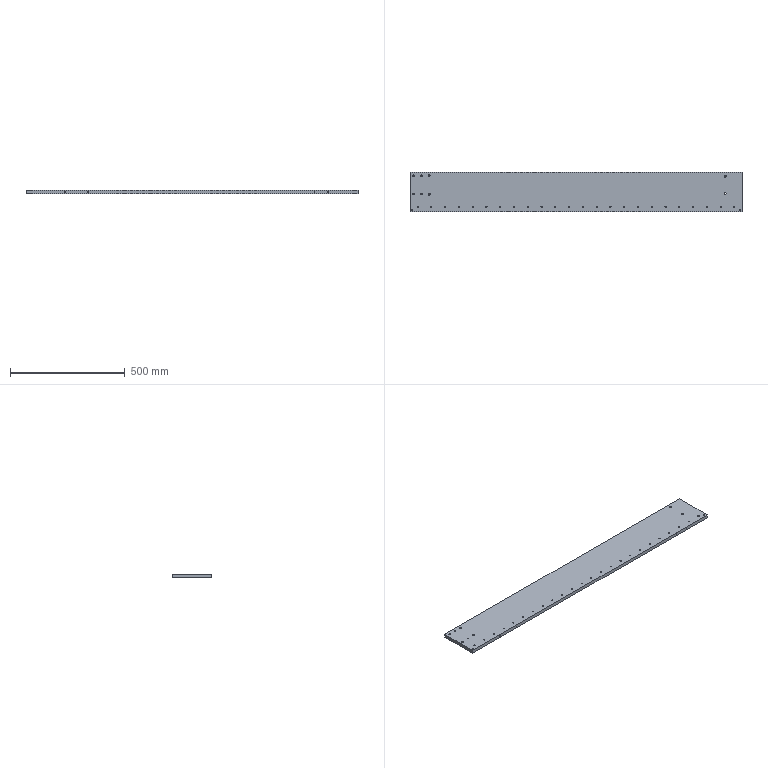Part | NX | 1 solid | 52 faces | box 1446 x 172 x 15 mm | volume 3717591 mm3 | cylinder 38 | cone 8 | plane 6 | commonest cylinder face diameters 5 x24 2.5 x4 6.8 x4 8.5 x4 3 x2
STEP:
#1=CARTESIAN_POINT('',(723.,-86.,0.));
#2=VERTEX_POINT('',#1);
#3=CARTESIAN_POINT('',(723.,86.,0.));
#4=VERTEX_POINT('',#3);
#5=CARTESIAN_POINT('',(723.,-86.,0.));
#6=DIRECTION('',(0.,1.,0.));
#7=VECTOR('',#6,1000.);
#8=LINE('',#5,#7);
#9=EDGE_CURVE('',#2,#4,#8,.T.);
#10=ORIENTED_EDGE('',*,*,#9,.T.);
#11=CARTESIAN_POINT('',(723.,86.,15.));
#12=VERTEX_POINT('',#11);
#13=CARTESIAN_POINT('',(723.,86.,15.));
#14=DIRECTION('',(0.,0.,-1.));
#15=VECTOR('',#14,1000.);
#16=LINE('',#13,#15);
#17=EDGE_CURVE('',#12,#4,#16,.T.);
#18=ORIENTED_EDGE('',*,*,#17,.F.);
#19=CARTESIAN_POINT('',(723.,-86.,15.));
#20=VERTEX_POINT('',#19);
#21=CARTESIAN_POINT('',(723.,-86.,15.));
#22=DIRECTION('',(0.,1.,0.));
#23=VECTOR('',#22,1000.);
#24=LINE('',#21,#23);
#25=EDGE_CURVE('',#20,#12,#24,.T.);
#26=ORIENTED_EDGE('',*,*,#25,.F.);
#27=CARTESIAN_POINT('',(723.,-86.,15.));
#28=DIRECTION('',(0.,0.,-1.));
#29=VECTOR('',#28,1000.);
#30=LINE('',#27,#29);
#31=EDGE_CURVE('',#20,#2,#30,.T.);
#32=ORIENTED_EDGE('',*,*,#31,.T.);
#33=EDGE_LOOP('',(#10,#18,#26,#32));
#34=FACE_BOUND('',#33,.T.);
#35=CARTESIAN_POINT('',(723.,-86.,15.));
#36=DIRECTION('',(-1.,0.,0.));
#37=DIRECTION('',(0.,0.,1.));
#38=AXIS2_PLACEMENT_3D('',#35,#36,#37);
#39=PLANE('',#38);
#40=ADVANCED_FACE('',(#34),#39,.F.);
#41=CARTESIAN_POINT('',(-723.,86.,0.));
#42=VERTEX_POINT('',#41);
#43=CARTESIAN_POINT('',(-723.,86.,0.));
#44=DIRECTION('',(-1.,0.,0.));
#45=VECTOR('',#44,1000.);
#46=LINE('',#43,#45);
#47=EDGE_CURVE('',#4,#42,#46,.T.);
#48=ORIENTED_EDGE('',*,*,#47,.T.);
#49=CARTESIAN_POINT('',(-723.,86.,15.));
#50=VERTEX_POINT('',#49);
#51=CARTESIAN_POINT('',(-723.,86.,15.));
#52=DIRECTION('',(0.,0.,-1.));
#53=VECTOR('',#52,1000.);
#54=LINE('',#51,#53);
#55=EDGE_CURVE('',#50,#42,#54,.T.);
#56=ORIENTED_EDGE('',*,*,#55,.F.);
#57=CARTESIAN_POINT('',(-723.,86.,15.));
#58=DIRECTION('',(-1.,0.,0.));
#59=VECTOR('',#58,1000.);
#60=LINE('',#57,#59);
#61=EDGE_CURVE('',#12,#50,#60,.T.);
#62=ORIENTED_EDGE('',*,*,#61,.F.);
#63=ORIENTED_EDGE('',*,*,#17,.T.);
#64=EDGE_LOOP('',(#48,#56,#62,#63));
#65=FACE_BOUND('',#64,.T.);
#66=CARTESIAN_POINT('',(-723.,86.,15.));
#67=DIRECTION('',(0.,-1.,0.));
#68=DIRECTION('',(0.,0.,-1.));
#69=AXIS2_PLACEMENT_3D('',#66,#67,#68);
#70=PLANE('',#69);
#71=ADVANCED_FACE('',(#65),#70,.F.);
#72=CARTESIAN_POINT('',(-723.,-86.,0.));
#73=VERTEX_POINT('',#72);
#74=CARTESIAN_POINT('',(-723.,-86.,0.));
#75=DIRECTION('',(0.,-1.,0.));
#76=VECTOR('',#75,1000.);
#77=LINE('',#74,#76);
#78=EDGE_CURVE('',#42,#73,#77,.T.);
#79=ORIENTED_EDGE('',*,*,#78,.T.);
#80=CARTESIAN_POINT('',(-723.,-86.,15.));
#81=VERTEX_POINT('',#80);
#82=CARTESIAN_POINT('',(-723.,-86.,15.));
#83=DIRECTION('',(0.,0.,-1.));
#84=VECTOR('',#83,1000.);
#85=LINE('',#82,#84);
#86=EDGE_CURVE('',#81,#73,#85,.T.);
#87=ORIENTED_EDGE('',*,*,#86,.F.);
#88=CARTESIAN_POINT('',(-723.,-86.,15.));
#89=DIRECTION('',(0.,-1.,0.));
#90=VECTOR('',#89,1000.);
#91=LINE('',#88,#90);
#92=EDGE_CURVE('',#50,#81,#91,.T.);
#93=ORIENTED_EDGE('',*,*,#92,.F.);
#94=ORIENTED_EDGE('',*,*,#55,.T.);
#95=EDGE_LOOP('',(#79,#87,#93,#94));
#96=FACE_BOUND('',#95,.T.);
#97=CARTESIAN_POINT('',(-723.,-86.,15.));
#98=DIRECTION('',(1.,0.,0.));
#99=DIRECTION('',(0.,0.,-1.));
#100=AXIS2_PLACEMENT_3D('',#97,#98,#99);
#101=PLANE('',#100);
#102=ADVANCED_FACE('',(#96),#101,.F.);
#103=CARTESIAN_POINT('',(593.,-86.,6.25));
#104=VERTEX_POINT('',#103);
#105=CARTESIAN_POINT('',(593.,-86.,7.5));
#106=DIRECTION('',(0.,-1.,0.));
#107=DIRECTION('',(0.,0.,-1.));
#108=AXIS2_PLACEMENT_3D('',#105,#106,#107);
#109=CIRCLE('',#108,1.25);
#110=EDGE_CURVE('',#104,#104,#109,.T.);
#111=ORIENTED_EDGE('',*,*,#110,.F.);
#112=EDGE_LOOP('',(#111));
#113=FACE_BOUND('',#112,.T.);
#114=CARTESIAN_POINT('',(533.,-86.,6.25));
#115=VERTEX_POINT('',#114);
#116=CARTESIAN_POINT('',(533.,-86.,7.5));
#117=DIRECTION('',(0.,-1.,0.));
#118=DIRECTION('',(0.,0.,-1.));
#119=AXIS2_PLACEMENT_3D('',#116,#117,#118);
#120=CIRCLE('',#119,1.25);
#121=EDGE_CURVE('',#115,#115,#120,.T.);
#122=ORIENTED_EDGE('',*,*,#121,.F.);
#123=EDGE_LOOP('',(#122));
#124=FACE_BOUND('',#123,.T.);
#125=CARTESIAN_POINT('',(-554.,-86.,6.25));
#126=VERTEX_POINT('',#125);
#127=CARTESIAN_POINT('',(-554.,-86.,7.5));
#128=DIRECTION('',(0.,-1.,0.));
#129=DIRECTION('',(0.,0.,-1.));
#130=AXIS2_PLACEMENT_3D('',#127,#128,#129);
#131=CIRCLE('',#130,1.25);
#132=EDGE_CURVE('',#126,#126,#131,.T.);
#133=ORIENTED_EDGE('',*,*,#132,.F.);
#134=EDGE_LOOP('',(#133));
#135=FACE_BOUND('',#134,.T.);
#136=CARTESIAN_POINT('',(-454.,-86.,6.25));
#137=VERTEX_POINT('',#136);
#138=CARTESIAN_POINT('',(-454.,-86.,7.5));
#139=DIRECTION('',(0.,-1.,0.));
#140=DIRECTION('',(0.,0.,-1.));
#141=AXIS2_PLACEMENT_3D('',#138,#139,#140);
#142=CIRCLE('',#141,1.25);
#143=EDGE_CURVE('',#137,#137,#142,.T.);
#144=ORIENTED_EDGE('',*,*,#143,.F.);
#145=EDGE_LOOP('',(#144));
#146=FACE_BOUND('',#145,.T.);
#147=CARTESIAN_POINT('',(-723.,-86.,0.));
#148=DIRECTION('',(1.,0.,0.));
#149=VECTOR('',#148,1000.);
#150=LINE('',#147,#149);
#151=EDGE_CURVE('',#73,#2,#150,.T.);
#152=ORIENTED_EDGE('',*,*,#151,.T.);
#153=ORIENTED_EDGE('',*,*,#31,.F.);
#154=CARTESIAN_POINT('',(-723.,-86.,15.));
#155=DIRECTION('',(1.,0.,0.));
#156=VECTOR('',#155,1000.);
#157=LINE('',#154,#156);
#158=EDGE_CURVE('',#81,#20,#157,.T.);
#159=ORIENTED_EDGE('',*,*,#158,.F.);
#160=ORIENTED_EDGE('',*,*,#86,.T.);
#161=EDGE_LOOP('',(#152,#153,#159,#160));
#162=FACE_BOUND('',#161,.T.);
#163=CARTESIAN_POINT('',(-723.,-86.,15.));
#164=DIRECTION('',(0.,1.,0.));
#165=DIRECTION('',(0.,0.,1.));
#166=AXIS2_PLACEMENT_3D('',#163,#164,#165);
#167=PLANE('',#166);
#168=ADVANCED_FACE('',(#113,#124,#135,#146,#162),#167,.F.);
#169=CARTESIAN_POINT('',(710.5,-77.5,15.));
#170=VERTEX_POINT('',#169);
#171=CARTESIAN_POINT('',(713.,-77.5,15.));
#172=DIRECTION('',(0.,0.,-1.));
#173=DIRECTION('',(-1.,0.,0.));
#174=AXIS2_PLACEMENT_3D('',#171,#172,#173);
#175=CIRCLE('',#174,2.5);
#176=EDGE_CURVE('',#170,#170,#175,.T.);
#177=ORIENTED_EDGE('',*,*,#176,.T.);
#178=EDGE_LOOP('',(#177));
#179=FACE_BOUND('',#178,.T.);
#180=CARTESIAN_POINT('',(-715.5,-77.5,15.));
#181=VERTEX_POINT('',#180);
#182=CARTESIAN_POINT('',(-713.,-77.5,15.));
#183=DIRECTION('',(0.,0.,-1.));
#184=DIRECTION('',(-1.,0.,0.));
#185=AXIS2_PLACEMENT_3D('',#182,#183,#184);
#186=CIRCLE('',#185,2.5);
#187=EDGE_CURVE('',#181,#181,#186,.T.);
#188=ORIENTED_EDGE('',*,*,#187,.T.);
#189=EDGE_LOOP('',(#188));
#190=FACE_BOUND('',#189,.T.);
#191=CARTESIAN_POINT('',(654.25,68.5,15.));
#192=VERTEX_POINT('',#191);
#193=CARTESIAN_POINT('',(650.,68.5,15.));
#194=DIRECTION('',(0.,0.,1.));
#195=DIRECTION('',(1.,0.,0.));
#196=AXIS2_PLACEMENT_3D('',#193,#194,#195);
#197=CIRCLE('',#196,4.25);
#198=EDGE_CURVE('',#192,#192,#197,.T.);
#199=ORIENTED_EDGE('',*,*,#198,.F.);
#200=EDGE_LOOP('',(#199));
#201=FACE_BOUND('',#200,.T.);
#202=CARTESIAN_POINT('',(654.25,-6.5,15.));
#203=VERTEX_POINT('',#202);
#204=CARTESIAN_POINT('',(650.,-6.5,15.));
#205=DIRECTION('',(0.,0.,1.));
#206=DIRECTION('',(1.,0.,0.));
#207=AXIS2_PLACEMENT_3D('',#204,#205,#206);
#208=CIRCLE('',#207,4.25);
#209=EDGE_CURVE('',#203,#203,#208,.T.);
#210=ORIENTED_EDGE('',*,*,#209,.F.);
#211=EDGE_LOOP('',(#210));
#212=FACE_BOUND('',#211,.T.);
#213=CARTESIAN_POINT('',(-635.75,71.,15.));
#214=VERTEX_POINT('',#213);
#215=CARTESIAN_POINT('',(-640.,71.,15.));
#216=DIRECTION('',(0.,0.,1.));
#217=DIRECTION('',(1.,0.,0.));
#218=AXIS2_PLACEMENT_3D('',#215,#216,#217);
#219=CIRCLE('',#218,4.25);
#220=EDGE_CURVE('',#214,#214,#219,.T.);
#221=ORIENTED_EDGE('',*,*,#220,.F.);
#222=EDGE_LOOP('',(#221));
#223=FACE_BOUND('',#222,.T.);
#224=CARTESIAN_POINT('',(-635.75,-9.,15.));
#225=VERTEX_POINT('',#224);
#226=CARTESIAN_POINT('',(-640.,-9.,15.));
#227=DIRECTION('',(0.,0.,1.));
#228=DIRECTION('',(1.,0.,0.));
#229=AXIS2_PLACEMENT_3D('',#226,#227,#228);
#230=CIRCLE('',#229,4.25);
#231=EDGE_CURVE('',#225,#225,#230,.T.);
#232=ORIENTED_EDGE('',*,*,#231,.F.);
#233=EDGE_LOOP('',(#232));
#234=FACE_BOUND('',#233,.T.);
#235=CARTESIAN_POINT('',(-704.6,-9.,15.));
#236=VERTEX_POINT('',#235);
#237=CARTESIAN_POINT('',(-708.,-9.,15.));
#238=DIRECTION('',(0.,0.,1.));
#239=DIRECTION('',(1.,0.,0.));
#240=AXIS2_PLACEMENT_3D('',#237,#238,#239);
#241=CIRCLE('',#240,3.4);
#242=EDGE_CURVE('',#236,#236,#241,.T.);
#243=ORIENTED_EDGE('',*,*,#242,.F.);
#244=EDGE_LOOP('',(#243));
#245=FACE_BOUND('',#244,.T.);
#246=CARTESIAN_POINT('',(-669.6,-9.,15.));
#247=VERTEX_POINT('',#246);
#248=CARTESIAN_POINT('',(-673.,-9.,15.));
#249=DIRECTION('',(0.,0.,1.));
#250=DIRECTION('',(1.,0.,0.));
#251=AXIS2_PLACEMENT_3D('',#248,#249,#250);
#252=CIRCLE('',#251,3.4);
#253=EDGE_CURVE('',#247,#247,#252,.T.);
#254=ORIENTED_EDGE('',*,*,#253,.F.);
#255=EDGE_LOOP('',(#254));
#256=FACE_BOUND('',#255,.T.);
#257=CARTESIAN_POINT('',(-704.6,71.,15.));
#258=VERTEX_POINT('',#257);
#259=CARTESIAN_POINT('',(-708.,71.,15.));
#260=DIRECTION('',(0.,0.,1.));
#261=DIRECTION('',(1.,0.,0.));
#262=AXIS2_PLACEMENT_3D('',#259,#260,#261);
#263=CIRCLE('',#262,3.4);
#264=EDGE_CURVE('',#258,#258,#263,.T.);
#265=ORIENTED_EDGE('',*,*,#264,.F.);
#266=EDGE_LOOP('',(#265));
#267=FACE_BOUND('',#266,.T.);
#268=CARTESIAN_POINT('',(-669.6,71.,15.));
#269=VERTEX_POINT('',#268);
#270=CARTESIAN_POINT('',(-673.,71.,15.));
#271=DIRECTION('',(0.,0.,1.));
#272=DIRECTION('',(1.,0.,0.));
#273=AXIS2_PLACEMENT_3D('',#270,#271,#272);
#274=CIRCLE('',#273,3.4);
#275=EDGE_CURVE('',#269,#269,#274,.T.);
#276=ORIENTED_EDGE('',*,*,#275,.F.);
#277=EDGE_LOOP('',(#276));
#278=FACE_BOUND('',#277,.T.);
#279=CARTESIAN_POINT('',(-627.5,-64.5,15.));
#280=VERTEX_POINT('',#279);
#281=CARTESIAN_POINT('',(-630.,-64.5,15.));
#282=DIRECTION('',(0.,0.,1.));
#283=DIRECTION('',(1.,0.,0.));
#284=AXIS2_PLACEMENT_3D('',#281,#282,#283);
#285=CIRCLE('',#284,2.5);
#286=EDGE_CURVE('',#280,#280,#285,.T.);
#287=ORIENTED_EDGE('',*,*,#286,.F.);
#288=EDGE_LOOP('',(#287));
#289=FACE_BOUND('',#288,.T.);
#290=CARTESIAN_POINT('',(-687.5,-64.5,15.));
#291=VERTEX_POINT('',#290);
#292=CARTESIAN_POINT('',(-690.,-64.5,15.));
#293=DIRECTION('',(0.,0.,1.));
#294=DIRECTION('',(1.,0.,0.));
#295=AXIS2_PLACEMENT_3D('',#292,#293,#294);
#296=CIRCLE('',#295,2.5);
#297=EDGE_CURVE('',#291,#291,#296,.T.);
#298=ORIENTED_EDGE('',*,*,#297,.F.);
#299=EDGE_LOOP('',(#298));
#300=FACE_BOUND('',#299,.T.);
#301=ORIENTED_EDGE('',*,*,#25,.T.);
#302=ORIENTED_EDGE('',*,*,#61,.T.);
#303=ORIENTED_EDGE('',*,*,#92,.T.);
#304=ORIENTED_EDGE('',*,*,#158,.T.);
#305=EDGE_LOOP('',(#301,#302,#303,#304));
#306=FACE_BOUND('',#305,.T.);
#307=CARTESIAN_POINT('',(-567.5,-64.5,15.));
#308=VERTEX_POINT('',#307);
#309=CARTESIAN_POINT('',(-570.,-64.5,15.));
#310=DIRECTION('',(0.,0.,1.));
#311=DIRECTION('',(1.,0.,0.));
#312=AXIS2_PLACEMENT_3D('',#309,#310,#311);
#313=CIRCLE('',#312,2.5);
#314=EDGE_CURVE('',#308,#308,#313,.T.);
#315=ORIENTED_EDGE('',*,*,#314,.F.);
#316=EDGE_LOOP('',(#315));
#317=FACE_BOUND('',#316,.T.);
#318=CARTESIAN_POINT('',(-507.5,-64.5,15.));
#319=VERTEX_POINT('',#318);
#320=CARTESIAN_POINT('',(-510.,-64.5,15.));
#321=DIRECTION('',(0.,0.,1.));
#322=DIRECTION('',(1.,0.,0.));
#323=AXIS2_PLACEMENT_3D('',#320,#321,#322);
#324=CIRCLE('',#323,2.5);
#325=EDGE_CURVE('',#319,#319,#324,.T.);
#326=ORIENTED_EDGE('',*,*,#325,.F.);
#327=EDGE_LOOP('',(#326));
#328=FACE_BOUND('',#327,.T.);
#329=CARTESIAN_POINT('',(-447.5,-64.5,15.));
#330=VERTEX_POINT('',#329);
#331=CARTESIAN_POINT('',(-450.,-64.5,15.));
#332=DIRECTION('',(0.,0.,1.));
#333=DIRECTION('',(1.,0.,0.));
#334=AXIS2_PLACEMENT_3D('',#331,#332,#333);
#335=CIRCLE('',#334,2.5);
#336=EDGE_CURVE('',#330,#330,#335,.T.);
#337=ORIENTED_EDGE('',*,*,#336,.F.);
#338=EDGE_LOOP('',(#337));
#339=FACE_BOUND('',#338,.T.);
#340=CARTESIAN_POINT('',(-387.5,-64.5,15.));
#341=VERTEX_POINT('',#340);
#342=CARTESIAN_POINT('',(-390.,-64.5,15.));
#343=DIRECTION('',(0.,0.,1.));
#344=DIRECTION('',(1.,0.,0.));
#345=AXIS2_PLACEMENT_3D('',#342,#343,#344);
#346=CIRCLE('',#345,2.5);
#347=EDGE_CURVE('',#341,#341,#346,.T.);
#348=ORIENTED_EDGE('',*,*,#347,.F.);
#349=EDGE_LOOP('',(#348));
#350=FACE_BOUND('',#349,.T.);
#351=CARTESIAN_POINT('',(-327.5,-64.5,15.));
#352=VERTEX_POINT('',#351);
#353=CARTESIAN_POINT('',(-330.,-64.5,15.));
#354=DIRECTION('',(0.,0.,1.));
#355=DIRECTION('',(1.,0.,0.));
#356=AXIS2_PLACEMENT_3D('',#353,#354,#355);
#357=CIRCLE('',#356,2.5);
#358=EDGE_CURVE('',#352,#352,#357,.T.);
#359=ORIENTED_EDGE('',*,*,#358,.F.);
#360=EDGE_LOOP('',(#359));
#361=FACE_BOUND('',#360,.T.);
#362=CARTESIAN_POINT('',(-267.5,-64.5,15.));
#363=VERTEX_POINT('',#362);
#364=CARTESIAN_POINT('',(-270.,-64.5,15.));
#365=DIRECTION('',(0.,0.,1.));
#366=DIRECTION('',(1.,0.,0.));
#367=AXIS2_PLACEMENT_3D('',#364,#365,#366);
#368=CIRCLE('',#367,2.5);
#369=EDGE_CURVE('',#363,#363,#368,.T.);
#370=ORIENTED_EDGE('',*,*,#369,.F.);
#371=EDGE_LOOP('',(#370));
#372=FACE_BOUND('',#371,.T.);
#373=CARTESIAN_POINT('',(-207.5,-64.5,15.));
#374=VERTEX_POINT('',#373);
#375=CARTESIAN_POINT('',(-210.,-64.5,15.));
#376=DIRECTION('',(0.,0.,1.));
#377=DIRECTION('',(1.,0.,0.));
#378=AXIS2_PLACEMENT_3D('',#375,#376,#377);
#379=CIRCLE('',#378,2.5);
#380=EDGE_CURVE('',#374,#374,#379,.T.);
#381=ORIENTED_EDGE('',*,*,#380,.F.);
#382=EDGE_LOOP('',(#381));
#383=FACE_BOUND('',#382,.T.);
#384=CARTESIAN_POINT('',(-147.5,-64.5,15.));
#385=VERTEX_POINT('',#384);
#386=CARTESIAN_POINT('',(-150.,-64.5,15.));
#387=DIRECTION('',(0.,0.,1.));
#388=DIRECTION('',(1.,0.,0.));
#389=AXIS2_PLACEMENT_3D('',#386,#387,#388);
#390=CIRCLE('',#389,2.5);
#391=EDGE_CURVE('',#385,#385,#390,.T.);
#392=ORIENTED_EDGE('',*,*,#391,.F.);
#393=EDGE_LOOP('',(#392));
#394=FACE_BOUND('',#393,.T.);
#395=CARTESIAN_POINT('',(-87.5,-64.5,15.));
#396=VERTEX_POINT('',#395);
#397=CARTESIAN_POINT('',(-90.,-64.5,15.));
#398=DIRECTION('',(0.,0.,1.));
#399=DIRECTION('',(1.,0.,0.));
#400=AXIS2_PLACEMENT_3D('',#397,#398,#399);
#401=CIRCLE('',#400,2.5);
#402=EDGE_CURVE('',#396,#396,#401,.T.);
#403=ORIENTED_EDGE('',*,*,#402,.F.);
#404=EDGE_LOOP('',(#403));
#405=FACE_BOUND('',#404,.T.);
#406=CARTESIAN_POINT('',(-27.5,-64.5,15.));
#407=VERTEX_POINT('',#406);
#408=CARTESIAN_POINT('',(-30.,-64.5,15.));
#409=DIRECTION('',(0.,0.,1.));
#410=DIRECTION('',(1.,0.,0.));
#411=AXIS2_PLACEMENT_3D('',#408,#409,#410);
#412=CIRCLE('',#411,2.5);
#413=EDGE_CURVE('',#407,#407,#412,.T.);
#414=ORIENTED_EDGE('',*,*,#413,.F.);
#415=EDGE_LOOP('',(#414));
#416=FACE_BOUND('',#415,.T.);
#417=CARTESIAN_POINT('',(32.5,-64.5,15.));
#418=VERTEX_POINT('',#417);
#419=CARTESIAN_POINT('',(30.,-64.5,15.));
#420=DIRECTION('',(0.,0.,1.));
#421=DIRECTION('',(1.,0.,0.));
#422=AXIS2_PLACEMENT_3D('',#419,#420,#421);
#423=CIRCLE('',#422,2.5);
#424=EDGE_CURVE('',#418,#418,#423,.T.);
#425=ORIENTED_EDGE('',*,*,#424,.F.);
#426=EDGE_LOOP('',(#425));
#427=FACE_BOUND('',#426,.T.);
#428=CARTESIAN_POINT('',(92.5,-64.5,15.));
#429=VERTEX_POINT('',#428);
#430=CARTESIAN_POINT('',(90.,-64.5,15.));
#431=DIRECTION('',(0.,0.,1.));
#432=DIRECTION('',(1.,0.,0.));
#433=AXIS2_PLACEMENT_3D('',#430,#431,#432);
#434=CIRCLE('',#433,2.5);
#435=EDGE_CURVE('',#429,#429,#434,.T.);
#436=ORIENTED_EDGE('',*,*,#435,.F.);
#437=EDGE_LOOP('',(#436));
#438=FACE_BOUND('',#437,.T.);
#439=CARTESIAN_POINT('',(152.5,-64.5,15.));
#440=VERTEX_POINT('',#439);
#441=CARTESIAN_POINT('',(150.,-64.5,15.));
#442=DIRECTION('',(0.,0.,1.));
#443=DIRECTION('',(1.,0.,0.));
#444=AXIS2_PLACEMENT_3D('',#441,#442,#443);
#445=CIRCLE('',#444,2.5);
#446=EDGE_CURVE('',#440,#440,#445,.T.);
#447=ORIENTED_EDGE('',*,*,#446,.F.);
#448=EDGE_LOOP('',(#447));
#449=FACE_BOUND('',#448,.T.);
#450=CARTESIAN_POINT('',(212.5,-64.5,15.));
#451=VERTEX_POINT('',#450);
#452=CARTESIAN_POINT('',(210.,-64.5,15.));
#453=DIRECTION('',(0.,0.,1.));
#454=DIRECTION('',(1.,0.,0.));
#455=AXIS2_PLACEMENT_3D('',#452,#453,#454);
#456=CIRCLE('',#455,2.5);
#457=EDGE_CURVE('',#451,#451,#456,.T.);
#458=ORIENTED_EDGE('',*,*,#457,.F.);
#459=EDGE_LOOP('',(#458));
#460=FACE_BOUND('',#459,.T.);
#461=CARTESIAN_POINT('',(272.5,-64.5,15.));
#462=VERTEX_POINT('',#461);
#463=CARTESIAN_POINT('',(270.,-64.5,15.));
#464=DIRECTION('',(0.,0.,1.));
#465=DIRECTION('',(1.,0.,0.));
#466=AXIS2_PLACEMENT_3D('',#463,#464,#465);
#467=CIRCLE('',#466,2.5);
#468=EDGE_CURVE('',#462,#462,#467,.T.);
#469=ORIENTED_EDGE('',*,*,#468,.F.);
#470=EDGE_LOOP('',(#469));
#471=FACE_BOUND('',#470,.T.);
#472=CARTESIAN_POINT('',(332.5,-64.5,15.));
#473=VERTEX_POINT('',#472);
#474=CARTESIAN_POINT('',(330.,-64.5,15.));
#475=DIRECTION('',(0.,0.,1.));
#476=DIRECTION('',(1.,0.,0.));
#477=AXIS2_PLACEMENT_3D('',#474,#475,#476);
#478=CIRCLE('',#477,2.5);
#479=EDGE_CURVE('',#473,#473,#478,.T.);
#480=ORIENTED_EDGE('',*,*,#479,.F.);
#481=EDGE_LOOP('',(#480));
#482=FACE_BOUND('',#481,.T.);
#483=CARTESIAN_POINT('',(392.5,-64.5,15.));
#484=VERTEX_POINT('',#483);
#485=CARTESIAN_POINT('',(390.,-64.5,15.));
#486=DIRECTION('',(0.,0.,1.));
#487=DIRECTION('',(1.,0.,0.));
#488=AXIS2_PLACEMENT_3D('',#485,#486,#487);
#489=CIRCLE('',#488,2.5);
#490=EDGE_CURVE('',#484,#484,#489,.T.);
#491=ORIENTED_EDGE('',*,*,#490,.F.);
#492=EDGE_LOOP('',(#491));
#493=FACE_BOUND('',#492,.T.);
#494=CARTESIAN_POINT('',(452.5,-64.5,15.));
#495=VERTEX_POINT('',#494);
#496=CARTESIAN_POINT('',(450.,-64.5,15.));
#497=DIRECTION('',(0.,0.,1.));
#498=DIRECTION('',(1.,0.,0.));
#499=AXIS2_PLACEMENT_3D('',#496,#497,#498);
#500=CIRCLE('',#499,2.5);
#501=EDGE_CURVE('',#495,#495,#500,.T.);
#502=ORIENTED_EDGE('',*,*,#501,.F.);
#503=EDGE_LOOP('',(#502));
#504=FACE_BOUND('',#503,.T.);
#505=CARTESIAN_POINT('',(512.5,-64.5,15.));
#506=VERTEX_POINT('',#505);
#507=CARTESIAN_POINT('',(510.,-64.5,15.));
#508=DIRECTION('',(0.,0.,1.));
#509=DIRECTION('',(1.,0.,0.));
#510=AXIS2_PLACEMENT_3D('',#507,#508,#509);
#511=CIRCLE('',#510,2.5);
#512=EDGE_CURVE('',#506,#506,#511,.T.);
#513=ORIENTED_EDGE('',*,*,#512,.F.);
#514=EDGE_LOOP('',(#513));
#515=FACE_BOUND('',#514,.T.);
#516=CARTESIAN_POINT('',(572.5,-64.5,15.));
#517=VERTEX_POINT('',#516);
#518=CARTESIAN_POINT('',(570.,-64.5,15.));
#519=DIRECTION('',(0.,0.,1.));
#520=DIRECTION('',(1.,0.,0.));
#521=AXIS2_PLACEMENT_3D('',#518,#519,#520);
#522=CIRCLE('',#521,2.5);
#523=EDGE_CURVE('',#517,#517,#522,.T.);
#524=ORIENTED_EDGE('',*,*,#523,.F.);
#525=EDGE_LOOP('',(#524));
#526=FACE_BOUND('',#525,.T.);
#527=CARTESIAN_POINT('',(632.5,-64.5,15.));
#528=VERTEX_POINT('',#527);
#529=CARTESIAN_POINT('',(630.,-64.5,15.));
#530=DIRECTION('',(0.,0.,1.));
#531=DIRECTION('',(1.,0.,0.));
#532=AXIS2_PLACEMENT_3D('',#529,#530,#531);
#533=CIRCLE('',#532,2.5);
#534=EDGE_CURVE('',#528,#528,#533,.T.);
#535=ORIENTED_EDGE('',*,*,#534,.F.);
#536=EDGE_LOOP('',(#535));
#537=FACE_BOUND('',#536,.T.);
#538=CARTESIAN_POINT('',(692.5,-64.5,15.));
#539=VERTEX_POINT('',#538);
#540=CARTESIAN_POINT('',(690.,-64.5,15.));
#541=DIRECTION('',(0.,0.,1.));
#542=DIRECTION('',(1.,0.,0.));
#543=AXIS2_PLACEMENT_3D('',#540,#541,#542);
#544=CIRCLE('',#543,2.5);
#545=EDGE_CURVE('',#539,#539,#544,.T.);
#546=ORIENTED_EDGE('',*,*,#545,.F.);
#547=EDGE_LOOP('',(#546));
#548=FACE_BOUND('',#547,.T.);
#549=CARTESIAN_POINT('',(0.,0.,15.));
#550=DIRECTION('',(0.,0.,-1.));
#551=DIRECTION('',(-1.,0.,0.));
#552=AXIS2_PLACEMENT_3D('',#549,#550,#551);
#553=PLANE('',#552);
#554=ADVANCED_FACE('',(#179,#190,#201,#212,#223,#234,#245,#256,#267,#278,#289,#300,#306,#317,#328,#339,#350,#361,#372,#383,#394,#405,#416,#427,#438,#449,#460,#471,#482,#493,#504,#515,#526,#537,#548),#553,.F.);
#555=CARTESIAN_POINT('',(710.5,-77.5,0.));
#556=VERTEX_POINT('',#555);
#557=CARTESIAN_POINT('',(713.,-77.5,0.));
#558=DIRECTION('',(0.,0.,-1.));
#559=DIRECTION('',(-1.,0.,0.));
#560=AXIS2_PLACEMENT_3D('',#557,#558,#559);
#561=CIRCLE('',#560,2.5);
#562=EDGE_CURVE('',#556,#556,#561,.F.);
#563=ORIENTED_EDGE('',*,*,#562,.T.);
#564=EDGE_LOOP('',(#563));
#565=FACE_BOUND('',#564,.T.);
#566=CARTESIAN_POINT('',(-715.5,-77.5,0.));
#567=VERTEX_POINT('',#566);
#568=CARTESIAN_POINT('',(-713.,-77.5,0.));
#569=DIRECTION('',(0.,0.,-1.));
#570=DIRECTION('',(-1.,0.,0.));
#571=AXIS2_PLACEMENT_3D('',#568,#569,#570);
#572=CIRCLE('',#571,2.5);
#573=EDGE_CURVE('',#567,#567,#572,.F.);
#574=ORIENTED_EDGE('',*,*,#573,.T.);
#575=EDGE_LOOP('',(#574));
#576=FACE_BOUND('',#575,.T.);
#577=CARTESIAN_POINT('',(645.75,68.5,0.));
#578=VERTEX_POINT('',#577);
#579=CARTESIAN_POINT('',(650.,68.5,0.));
#580=DIRECTION('',(0.,0.,-1.));
#581=DIRECTION('',(-1.,0.,0.));
#582=AXIS2_PLACEMENT_3D('',#579,#580,#581);
#583=CIRCLE('',#582,4.25);
#584=EDGE_CURVE('',#578,#578,#583,.T.);
#585=ORIENTED_EDGE('',*,*,#584,.F.);
#586=EDGE_LOOP('',(#585));
#587=FACE_BOUND('',#586,.T.);
#588=CARTESIAN_POINT('',(645.75,-6.5,0.));
#589=VERTEX_POINT('',#588);
#590=CARTESIAN_POINT('',(650.,-6.5,0.));
#591=DIRECTION('',(0.,0.,-1.));
#592=DIRECTION('',(-1.,0.,0.));
#593=AXIS2_PLACEMENT_3D('',#590,#591,#592);
#594=CIRCLE('',#593,4.25);
#595=EDGE_CURVE('',#589,#589,#594,.T.);
#596=ORIENTED_EDGE('',*,*,#595,.F.);
#597=EDGE_LOOP('',(#596));
#598=FACE_BOUND('',#597,.T.);
#599=CARTESIAN_POINT('',(-644.25,71.,0.));
#600=VERTEX_POINT('',#599);
#601=CARTESIAN_POINT('',(-640.,71.,0.));
#602=DIRECTION('',(0.,0.,-1.));
#603=DIRECTION('',(-1.,0.,0.));
#604=AXIS2_PLACEMENT_3D('',#601,#602,#603);
#605=CIRCLE('',#604,4.25);
#606=EDGE_CURVE('',#600,#600,#605,.T.);
#607=ORIENTED_EDGE('',*,*,#606,.F.);
#608=EDGE_LOOP('',(#607));
#609=FACE_BOUND('',#608,.T.);
#610=CARTESIAN_POINT('',(-644.25,-9.,0.));
#611=VERTEX_POINT('',#610);
#612=CARTESIAN_POINT('',(-640.,-9.,0.));
#613=DIRECTION('',(0.,0.,-1.));
#614=DIRECTION('',(-1.,0.,0.));
#615=AXIS2_PLACEMENT_3D('',#612,#613,#614);
#616=CIRCLE('',#615,4.25);
#617=EDGE_CURVE('',#611,#611,#616,.T.);
#618=ORIENTED_EDGE('',*,*,#617,.F.);
#619=EDGE_LOOP('',(#618));
#620=FACE_BOUND('',#619,.T.);
#621=CARTESIAN_POINT('',(-711.4,-9.,0.));
#622=VERTEX_POINT('',#621);
#623=CARTESIAN_POINT('',(-708.,-9.,0.));
#624=DIRECTION('',(0.,0.,-1.));
#625=DIRECTION('',(-1.,0.,0.));
#626=AXIS2_PLACEMENT_3D('',#623,#624,#625);
#627=CIRCLE('',#626,3.4);
#628=EDGE_CURVE('',#622,#622,#627,.T.);
#629=ORIENTED_EDGE('',*,*,#628,.F.);
#630=EDGE_LOOP('',(#629));
#631=FACE_BOUND('',#630,.T.);
#632=CARTESIAN_POINT('',(-676.4,-9.,0.));
#633=VERTEX_POINT('',#632);
#634=CARTESIAN_POINT('',(-673.,-9.,0.));
#635=DIRECTION('',(0.,0.,-1.));
#636=DIRECTION('',(-1.,0.,0.));
#637=AXIS2_PLACEMENT_3D('',#634,#635,#636);
#638=CIRCLE('',#637,3.4);
#639=EDGE_CURVE('',#633,#633,#638,.T.);
#640=ORIENTED_EDGE('',*,*,#639,.F.);
#641=EDGE_LOOP('',(#640));
#642=FACE_BOUND('',#641,.T.);
#643=CARTESIAN_POINT('',(-711.4,71.,0.));
#644=VERTEX_POINT('',#643);
#645=CARTESIAN_POINT('',(-708.,71.,0.));
#646=DIRECTION('',(0.,0.,-1.));
#647=DIRECTION('',(-1.,0.,0.));
#648=AXIS2_PLACEMENT_3D('',#645,#646,#647);
#649=CIRCLE('',#648,3.4);
#650=EDGE_CURVE('',#644,#644,#649,.T.);
#651=ORIENTED_EDGE('',*,*,#650,.F.);
#652=EDGE_LOOP('',(#651));
#653=FACE_BOUND('',#652,.T.);
#654=CARTESIAN_POINT('',(-676.4,71.,0.));
#655=VERTEX_POINT('',#654);
#656=CARTESIAN_POINT('',(-673.,71.,0.));
#657=DIRECTION('',(0.,0.,-1.));
#658=DIRECTION('',(-1.,0.,0.));
#659=AXIS2_PLACEMENT_3D('',#656,#657,#658);
#660=CIRCLE('',#659,3.4);
#661=EDGE_CURVE('',#655,#655,#660,.T.);
#662=ORIENTED_EDGE('',*,*,#661,.F.);
#663=EDGE_LOOP('',(#662));
#664=FACE_BOUND('',#663,.T.);
#665=CARTESIAN_POINT('',(-632.5,-64.5,0.));
#666=VERTEX_POINT('',#665);
#667=CARTESIAN_POINT('',(-630.,-64.5,0.));
#668=DIRECTION('',(0.,0.,-1.));
#669=DIRECTION('',(-1.,0.,0.));
#670=AXIS2_PLACEMENT_3D('',#667,#668,#669);
#671=CIRCLE('',#670,2.5);
#672=EDGE_CURVE('',#666,#666,#671,.T.);
#673=ORIENTED_EDGE('',*,*,#672,.F.);
#674=EDGE_LOOP('',(#673));
#675=FACE_BOUND('',#674,.T.);
#676=CARTESIAN_POINT('',(-692.5,-64.5,0.));
#677=VERTEX_POINT('',#676);
#678=CARTESIAN_POINT('',(-690.,-64.5,0.));
#679=DIRECTION('',(0.,0.,-1.));
#680=DIRECTION('',(-1.,0.,0.));
#681=AXIS2_PLACEMENT_3D('',#678,#679,#680);
#682=CIRCLE('',#681,2.5);
#683=EDGE_CURVE('',#677,#677,#682,.T.);
#684=ORIENTED_EDGE('',*,*,#683,.F.);
#685=EDGE_LOOP('',(#684));
#686=FACE_BOUND('',#685,.T.);
#687=ORIENTED_EDGE('',*,*,#9,.F.);
#688=ORIENTED_EDGE('',*,*,#151,.F.);
#689=ORIENTED_EDGE('',*,*,#78,.F.);
#690=ORIENTED_EDGE('',*,*,#47,.F.);
#691=EDGE_LOOP('',(#687,#688,#689,#690));
#692=FACE_BOUND('',#691,.T.);
#693=CARTESIAN_POINT('',(-572.5,-64.5,0.));
#694=VERTEX_POINT('',#693);
#695=CARTESIAN_POINT('',(-570.,-64.5,0.));
#696=DIRECTION('',(0.,0.,-1.));
#697=DIRECTION('',(-1.,0.,0.));
#698=AXIS2_PLACEMENT_3D('',#695,#696,#697);
#699=CIRCLE('',#698,2.5);
#700=EDGE_CURVE('',#694,#694,#699,.T.);
#701=ORIENTED_EDGE('',*,*,#700,.F.);
#702=EDGE_LOOP('',(#701));
#703=FACE_BOUND('',#702,.T.);
#704=CARTESIAN_POINT('',(-512.5,-64.5,0.));
#705=VERTEX_POINT('',#704);
#706=CARTESIAN_POINT('',(-510.,-64.5,0.));
#707=DIRECTION('',(0.,0.,-1.));
#708=DIRECTION('',(-1.,0.,0.));
#709=AXIS2_PLACEMENT_3D('',#706,#707,#708);
#710=CIRCLE('',#709,2.5);
#711=EDGE_CURVE('',#705,#705,#710,.T.);
#712=ORIENTED_EDGE('',*,*,#711,.F.);
#713=EDGE_LOOP('',(#712));
#714=FACE_BOUND('',#713,.T.);
#715=CARTESIAN_POINT('',(-452.5,-64.5,0.));
#716=VERTEX_POINT('',#715);
#717=CARTESIAN_POINT('',(-450.,-64.5,0.));
#718=DIRECTION('',(0.,0.,-1.));
#719=DIRECTION('',(-1.,0.,0.));
#720=AXIS2_PLACEMENT_3D('',#717,#718,#719);
#721=CIRCLE('',#720,2.5);
#722=EDGE_CURVE('',#716,#716,#721,.T.);
#723=ORIENTED_EDGE('',*,*,#722,.F.);
#724=EDGE_LOOP('',(#723));
#725=FACE_BOUND('',#724,.T.);
#726=CARTESIAN_POINT('',(-392.5,-64.5,0.));
#727=VERTEX_POINT('',#726);
#728=CARTESIAN_POINT('',(-390.,-64.5,0.));
#729=DIRECTION('',(0.,0.,-1.));
#730=DIRECTION('',(-1.,0.,0.));
#731=AXIS2_PLACEMENT_3D('',#728,#729,#730);
#732=CIRCLE('',#731,2.5);
#733=EDGE_CURVE('',#727,#727,#732,.T.);
#734=ORIENTED_EDGE('',*,*,#733,.F.);
#735=EDGE_LOOP('',(#734));
#736=FACE_BOUND('',#735,.T.);
#737=CARTESIAN_POINT('',(-332.5,-64.5,0.));
#738=VERTEX_POINT('',#737);
#739=CARTESIAN_POINT('',(-330.,-64.5,0.));
#740=DIRECTION('',(0.,0.,-1.));
#741=DIRECTION('',(-1.,0.,0.));
#742=AXIS2_PLACEMENT_3D('',#739,#740,#741);
#743=CIRCLE('',#742,2.5);
#744=EDGE_CURVE('',#738,#738,#743,.T.);
#745=ORIENTED_EDGE('',*,*,#744,.F.);
#746=EDGE_LOOP('',(#745));
#747=FACE_BOUND('',#746,.T.);
#748=CARTESIAN_POINT('',(-272.5,-64.5,0.));
#749=VERTEX_POINT('',#748);
#750=CARTESIAN_POINT('',(-270.,-64.5,0.));
#751=DIRECTION('',(0.,0.,-1.));
#752=DIRECTION('',(-1.,0.,0.));
#753=AXIS2_PLACEMENT_3D('',#750,#751,#752);
#754=CIRCLE('',#753,2.5);
#755=EDGE_CURVE('',#749,#749,#754,.T.);
#756=ORIENTED_EDGE('',*,*,#755,.F.);
#757=EDGE_LOOP('',(#756));
#758=FACE_BOUND('',#757,.T.);
#759=CARTESIAN_POINT('',(-212.5,-64.5,0.));
#760=VERTEX_POINT('',#759);
#761=CARTESIAN_POINT('',(-210.,-64.5,0.));
#762=DIRECTION('',(0.,0.,-1.));
#763=DIRECTION('',(-1.,0.,0.));
#764=AXIS2_PLACEMENT_3D('',#761,#762,#763);
#765=CIRCLE('',#764,2.5);
#766=EDGE_CURVE('',#760,#760,#765,.T.);
#767=ORIENTED_EDGE('',*,*,#766,.F.);
#768=EDGE_LOOP('',(#767));
#769=FACE_BOUND('',#768,.T.);
#770=CARTESIAN_POINT('',(-152.5,-64.5,0.));
#771=VERTEX_POINT('',#770);
#772=CARTESIAN_POINT('',(-150.,-64.5,0.));
#773=DIRECTION('',(0.,0.,-1.));
#774=DIRECTION('',(-1.,0.,0.));
#775=AXIS2_PLACEMENT_3D('',#772,#773,#774);
#776=CIRCLE('',#775,2.5);
#777=EDGE_CURVE('',#771,#771,#776,.T.);
#778=ORIENTED_EDGE('',*,*,#777,.F.);
#779=EDGE_LOOP('',(#778));
#780=FACE_BOUND('',#779,.T.);
#781=CARTESIAN_POINT('',(-92.5,-64.5,0.));
#782=VERTEX_POINT('',#781);
#783=CARTESIAN_POINT('',(-90.,-64.5,0.));
#784=DIRECTION('',(0.,0.,-1.));
#785=DIRECTION('',(-1.,0.,0.));
#786=AXIS2_PLACEMENT_3D('',#783,#784,#785);
#787=CIRCLE('',#786,2.5);
#788=EDGE_CURVE('',#782,#782,#787,.T.);
#789=ORIENTED_EDGE('',*,*,#788,.F.);
#790=EDGE_LOOP('',(#789));
#791=FACE_BOUND('',#790,.T.);
#792=CARTESIAN_POINT('',(-32.5,-64.5,0.));
#793=VERTEX_POINT('',#792);
#794=CARTESIAN_POINT('',(-30.,-64.5,0.));
#795=DIRECTION('',(0.,0.,-1.));
#796=DIRECTION('',(-1.,0.,0.));
#797=AXIS2_PLACEMENT_3D('',#794,#795,#796);
#798=CIRCLE('',#797,2.5);
#799=EDGE_CURVE('',#793,#793,#798,.T.);
#800=ORIENTED_EDGE('',*,*,#799,.F.);
#801=EDGE_LOOP('',(#800));
#802=FACE_BOUND('',#801,.T.);
#803=CARTESIAN_POINT('',(27.5,-64.5,0.));
#804=VERTEX_POINT('',#803);
#805=CARTESIAN_POINT('',(30.,-64.5,0.));
#806=DIRECTION('',(0.,0.,-1.));
#807=DIRECTION('',(-1.,0.,0.));
#808=AXIS2_PLACEMENT_3D('',#805,#806,#807);
#809=CIRCLE('',#808,2.5);
#810=EDGE_CURVE('',#804,#804,#809,.T.);
#811=ORIENTED_EDGE('',*,*,#810,.F.);
#812=EDGE_LOOP('',(#811));
#813=FACE_BOUND('',#812,.T.);
#814=CARTESIAN_POINT('',(87.5,-64.5,0.));
#815=VERTEX_POINT('',#814);
#816=CARTESIAN_POINT('',(90.,-64.5,0.));
#817=DIRECTION('',(0.,0.,-1.));
#818=DIRECTION('',(-1.,0.,0.));
#819=AXIS2_PLACEMENT_3D('',#816,#817,#818);
#820=CIRCLE('',#819,2.5);
#821=EDGE_CURVE('',#815,#815,#820,.T.);
#822=ORIENTED_EDGE('',*,*,#821,.F.);
#823=EDGE_LOOP('',(#822));
#824=FACE_BOUND('',#823,.T.);
#825=CARTESIAN_POINT('',(147.5,-64.5,0.));
#826=VERTEX_POINT('',#825);
#827=CARTESIAN_POINT('',(150.,-64.5,0.));
#828=DIRECTION('',(0.,0.,-1.));
#829=DIRECTION('',(-1.,0.,0.));
#830=AXIS2_PLACEMENT_3D('',#827,#828,#829);
#831=CIRCLE('',#830,2.5);
#832=EDGE_CURVE('',#826,#826,#831,.T.);
#833=ORIENTED_EDGE('',*,*,#832,.F.);
#834=EDGE_LOOP('',(#833));
#835=FACE_BOUND('',#834,.T.);
#836=CARTESIAN_POINT('',(207.5,-64.5,0.));
#837=VERTEX_POINT('',#836);
#838=CARTESIAN_POINT('',(210.,-64.5,0.));
#839=DIRECTION('',(0.,0.,-1.));
#840=DIRECTION('',(-1.,0.,0.));
#841=AXIS2_PLACEMENT_3D('',#838,#839,#840);
#842=CIRCLE('',#841,2.5);
#843=EDGE_CURVE('',#837,#837,#842,.T.);
#844=ORIENTED_EDGE('',*,*,#843,.F.);
#845=EDGE_LOOP('',(#844));
#846=FACE_BOUND('',#845,.T.);
#847=CARTESIAN_POINT('',(267.5,-64.5,0.));
#848=VERTEX_POINT('',#847);
#849=CARTESIAN_POINT('',(270.,-64.5,0.));
#850=DIRECTION('',(0.,0.,-1.));
#851=DIRECTION('',(-1.,0.,0.));
#852=AXIS2_PLACEMENT_3D('',#849,#850,#851);
#853=CIRCLE('',#852,2.5);
#854=EDGE_CURVE('',#848,#848,#853,.T.);
#855=ORIENTED_EDGE('',*,*,#854,.F.);
#856=EDGE_LOOP('',(#855));
#857=FACE_BOUND('',#856,.T.);
#858=CARTESIAN_POINT('',(327.5,-64.5,0.));
#859=VERTEX_POINT('',#858);
#860=CARTESIAN_POINT('',(330.,-64.5,0.));
#861=DIRECTION('',(0.,0.,-1.));
#862=DIRECTION('',(-1.,0.,0.));
#863=AXIS2_PLACEMENT_3D('',#860,#861,#862);
#864=CIRCLE('',#863,2.5);
#865=EDGE_CURVE('',#859,#859,#864,.T.);
#866=ORIENTED_EDGE('',*,*,#865,.F.);
#867=EDGE_LOOP('',(#866));
#868=FACE_BOUND('',#867,.T.);
#869=CARTESIAN_POINT('',(387.5,-64.5,0.));
#870=VERTEX_POINT('',#869);
#871=CARTESIAN_POINT('',(390.,-64.5,0.));
#872=DIRECTION('',(0.,0.,-1.));
#873=DIRECTION('',(-1.,0.,0.));
#874=AXIS2_PLACEMENT_3D('',#871,#872,#873);
#875=CIRCLE('',#874,2.5);
#876=EDGE_CURVE('',#870,#870,#875,.T.);
#877=ORIENTED_EDGE('',*,*,#876,.F.);
#878=EDGE_LOOP('',(#877));
#879=FACE_BOUND('',#878,.T.);
#880=CARTESIAN_POINT('',(447.5,-64.5,0.));
#881=VERTEX_POINT('',#880);
#882=CARTESIAN_POINT('',(450.,-64.5,0.));
#883=DIRECTION('',(0.,0.,-1.));
#884=DIRECTION('',(-1.,0.,0.));
#885=AXIS2_PLACEMENT_3D('',#882,#883,#884);
#886=CIRCLE('',#885,2.5);
#887=EDGE_CURVE('',#881,#881,#886,.T.);
#888=ORIENTED_EDGE('',*,*,#887,.F.);
#889=EDGE_LOOP('',(#888));
#890=FACE_BOUND('',#889,.T.);
#891=CARTESIAN_POINT('',(507.5,-64.5,0.));
#892=VERTEX_POINT('',#891);
#893=CARTESIAN_POINT('',(510.,-64.5,0.));
#894=DIRECTION('',(0.,0.,-1.));
#895=DIRECTION('',(-1.,0.,0.));
#896=AXIS2_PLACEMENT_3D('',#893,#894,#895);
#897=CIRCLE('',#896,2.5);
#898=EDGE_CURVE('',#892,#892,#897,.T.);
#899=ORIENTED_EDGE('',*,*,#898,.F.);
#900=EDGE_LOOP('',(#899));
#901=FACE_BOUND('',#900,.T.);
#902=CARTESIAN_POINT('',(567.5,-64.5,0.));
#903=VERTEX_POINT('',#902);
#904=CARTESIAN_POINT('',(570.,-64.5,0.));
#905=DIRECTION('',(0.,0.,-1.));
#906=DIRECTION('',(-1.,0.,0.));
#907=AXIS2_PLACEMENT_3D('',#904,#905,#906);
#908=CIRCLE('',#907,2.5);
#909=EDGE_CURVE('',#903,#903,#908,.T.);
#910=ORIENTED_EDGE('',*,*,#909,.F.);
#911=EDGE_LOOP('',(#910));
#912=FACE_BOUND('',#911,.T.);
#913=CARTESIAN_POINT('',(627.5,-64.5,0.));
#914=VERTEX_POINT('',#913);
#915=CARTESIAN_POINT('',(630.,-64.5,0.));
#916=DIRECTION('',(0.,0.,-1.));
#917=DIRECTION('',(-1.,0.,0.));
#918=AXIS2_PLACEMENT_3D('',#915,#916,#917);
#919=CIRCLE('',#918,2.5);
#920=EDGE_CURVE('',#914,#914,#919,.T.);
#921=ORIENTED_EDGE('',*,*,#920,.F.);
#922=EDGE_LOOP('',(#921));
#923=FACE_BOUND('',#922,.T.);
#924=CARTESIAN_POINT('',(687.5,-64.5,0.));
#925=VERTEX_POINT('',#924);
#926=CARTESIAN_POINT('',(690.,-64.5,0.));
#927=DIRECTION('',(0.,0.,-1.));
#928=DIRECTION('',(-1.,0.,0.));
#929=AXIS2_PLACEMENT_3D('',#926,#927,#928);
#930=CIRCLE('',#929,2.5);
#931=EDGE_CURVE('',#925,#925,#930,.T.);
#932=ORIENTED_EDGE('',*,*,#931,.F.);
#933=EDGE_LOOP('',(#932));
#934=FACE_BOUND('',#933,.T.);
#935=CARTESIAN_POINT('',(0.,0.,0.));
#936=DIRECTION('',(0.,0.,-1.));
#937=DIRECTION('',(-1.,0.,0.));
#938=AXIS2_PLACEMENT_3D('',#935,#936,#937);
#939=PLANE('',#938);
#940=ADVANCED_FACE('',(#565,#576,#587,#598,#609,#620,#631,#642,#653,#664,#675,#686,#692,#703,#714,#725,#736,#747,#758,#769,#780,#791,#802,#813,#824,#835,#846,#857,#868,#879,#890,#901,#912,#923,#934),#939,.T.);
#941=ORIENTED_EDGE('',*,*,#683,.T.);
#942=EDGE_LOOP('',(#941));
#943=FACE_BOUND('',#942,.T.);
#944=ORIENTED_EDGE('',*,*,#297,.T.);
#945=EDGE_LOOP('',(#944));
#946=FACE_BOUND('',#945,.T.);
#947=CARTESIAN_POINT('',(-690.,-64.5,15.));
#948=DIRECTION('',(0.,0.,1.));
#949=DIRECTION('',(1.,0.,0.));
#950=AXIS2_PLACEMENT_3D('',#947,#948,#949);
#951=CYLINDRICAL_SURFACE('',#950,2.5);
#952=ADVANCED_FACE('',(#943,#946),#951,.F.);
#953=ORIENTED_EDGE('',*,*,#672,.T.);
#954=EDGE_LOOP('',(#953));
#955=FACE_BOUND('',#954,.T.);
#956=ORIENTED_EDGE('',*,*,#286,.T.);
#957=EDGE_LOOP('',(#956));
#958=FACE_BOUND('',#957,.T.);
#959=CARTESIAN_POINT('',(-630.,-64.5,15.));
#960=DIRECTION('',(0.,0.,1.));
#961=DIRECTION('',(1.,0.,0.));
#962=AXIS2_PLACEMENT_3D('',#959,#960,#961);
#963=CYLINDRICAL_SURFACE('',#962,2.5);
#964=ADVANCED_FACE('',(#955,#958),#963,.F.);
#965=ORIENTED_EDGE('',*,*,#700,.T.);
#966=EDGE_LOOP('',(#965));
#967=FACE_BOUND('',#966,.T.);
#968=ORIENTED_EDGE('',*,*,#314,.T.);
#969=EDGE_LOOP('',(#968));
#970=FACE_BOUND('',#969,.T.);
#971=CARTESIAN_POINT('',(-570.,-64.5,15.));
#972=DIRECTION('',(0.,0.,1.));
#973=DIRECTION('',(1.,0.,0.));
#974=AXIS2_PLACEMENT_3D('',#971,#972,#973);
#975=CYLINDRICAL_SURFACE('',#974,2.5);
#976=ADVANCED_FACE('',(#967,#970),#975,.F.);
#977=ORIENTED_EDGE('',*,*,#711,.T.);
#978=EDGE_LOOP('',(#977));
#979=FACE_BOUND('',#978,.T.);
#980=ORIENTED_EDGE('',*,*,#325,.T.);
#981=EDGE_LOOP('',(#980));
#982=FACE_BOUND('',#981,.T.);
#983=CARTESIAN_POINT('',(-510.,-64.5,15.));
#984=DIRECTION('',(0.,0.,1.));
#985=DIRECTION('',(1.,0.,0.));
#986=AXIS2_PLACEMENT_3D('',#983,#984,#985);
#987=CYLINDRICAL_SURFACE('',#986,2.5);
#988=ADVANCED_FACE('',(#979,#982),#987,.F.);
#989=ORIENTED_EDGE('',*,*,#722,.T.);
#990=EDGE_LOOP('',(#989));
#991=FACE_BOUND('',#990,.T.);
#992=ORIENTED_EDGE('',*,*,#336,.T.);
#993=EDGE_LOOP('',(#992));
#994=FACE_BOUND('',#993,.T.);
#995=CARTESIAN_POINT('',(-450.,-64.5,15.));
#996=DIRECTION('',(0.,0.,1.));
#997=DIRECTION('',(1.,0.,0.));
#998=AXIS2_PLACEMENT_3D('',#995,#996,#997);
#999=CYLINDRICAL_SURFACE('',#998,2.5);
#1000=ADVANCED_FACE('',(#991,#994),#999,.F.);
#1001=ORIENTED_EDGE('',*,*,#733,.T.);
#1002=EDGE_LOOP('',(#1001));
#1003=FACE_BOUND('',#1002,.T.);
#1004=ORIENTED_EDGE('',*,*,#347,.T.);
#1005=EDGE_LOOP('',(#1004));
#1006=FACE_BOUND('',#1005,.T.);
#1007=CARTESIAN_POINT('',(-390.,-64.5,15.));
#1008=DIRECTION('',(0.,0.,1.));
#1009=DIRECTION('',(1.,0.,0.));
#1010=AXIS2_PLACEMENT_3D('',#1007,#1008,#1009);
#1011=CYLINDRICAL_SURFACE('',#1010,2.5);
#1012=ADVANCED_FACE('',(#1003,#1006),#1011,.F.);
#1013=ORIENTED_EDGE('',*,*,#744,.T.);
#1014=EDGE_LOOP('',(#1013));
#1015=FACE_BOUND('',#1014,.T.);
#1016=ORIENTED_EDGE('',*,*,#358,.T.);
#1017=EDGE_LOOP('',(#1016));
#1018=FACE_BOUND('',#1017,.T.);
#1019=CARTESIAN_POINT('',(-330.,-64.5,15.));
#1020=DIRECTION('',(0.,0.,1.));
#1021=DIRECTION('',(1.,0.,0.));
#1022=AXIS2_PLACEMENT_3D('',#1019,#1020,#1021);
#1023=CYLINDRICAL_SURFACE('',#1022,2.5);
#1024=ADVANCED_FACE('',(#1015,#1018),#1023,.F.);
#1025=ORIENTED_EDGE('',*,*,#755,.T.);
#1026=EDGE_LOOP('',(#1025));
#1027=FACE_BOUND('',#1026,.T.);
#1028=ORIENTED_EDGE('',*,*,#369,.T.);
#1029=EDGE_LOOP('',(#1028));
#1030=FACE_BOUND('',#1029,.T.);
#1031=CARTESIAN_POINT('',(-270.,-64.5,15.));
#1032=DIRECTION('',(0.,0.,1.));
#1033=DIRECTION('',(1.,0.,0.));
#1034=AXIS2_PLACEMENT_3D('',#1031,#1032,#1033);
#1035=CYLINDRICAL_SURFACE('',#1034,2.5);
#1036=ADVANCED_FACE('',(#1027,#1030),#1035,.F.);
#1037=ORIENTED_EDGE('',*,*,#766,.T.);
#1038=EDGE_LOOP('',(#1037));
#1039=FACE_BOUND('',#1038,.T.);
#1040=ORIENTED_EDGE('',*,*,#380,.T.);
#1041=EDGE_LOOP('',(#1040));
#1042=FACE_BOUND('',#1041,.T.);
#1043=CARTESIAN_POINT('',(-210.,-64.5,15.));
#1044=DIRECTION('',(0.,0.,1.));
#1045=DIRECTION('',(1.,0.,0.));
#1046=AXIS2_PLACEMENT_3D('',#1043,#1044,#1045);
#1047=CYLINDRICAL_SURFACE('',#1046,2.5);
#1048=ADVANCED_FACE('',(#1039,#1042),#1047,.F.);
#1049=ORIENTED_EDGE('',*,*,#777,.T.);
#1050=EDGE_LOOP('',(#1049));
#1051=FACE_BOUND('',#1050,.T.);
#1052=ORIENTED_EDGE('',*,*,#391,.T.);
#1053=EDGE_LOOP('',(#1052));
#1054=FACE_BOUND('',#1053,.T.);
#1055=CARTESIAN_POINT('',(-150.,-64.5,15.));
#1056=DIRECTION('',(0.,0.,1.));
#1057=DIRECTION('',(1.,0.,0.));
#1058=AXIS2_PLACEMENT_3D('',#1055,#1056,#1057);
#1059=CYLINDRICAL_SURFACE('',#1058,2.5);
#1060=ADVANCED_FACE('',(#1051,#1054),#1059,.F.);
#1061=ORIENTED_EDGE('',*,*,#788,.T.);
#1062=EDGE_LOOP('',(#1061));
#1063=FACE_BOUND('',#1062,.T.);
#1064=ORIENTED_EDGE('',*,*,#402,.T.);
#1065=EDGE_LOOP('',(#1064));
#1066=FACE_BOUND('',#1065,.T.);
#1067=CARTESIAN_POINT('',(-90.,-64.5,15.));
#1068=DIRECTION('',(0.,0.,1.));
#1069=DIRECTION('',(1.,0.,0.));
#1070=AXIS2_PLACEMENT_3D('',#1067,#1068,#1069);
#1071=CYLINDRICAL_SURFACE('',#1070,2.5);
#1072=ADVANCED_FACE('',(#1063,#1066),#1071,.F.);
#1073=ORIENTED_EDGE('',*,*,#799,.T.);
#1074=EDGE_LOOP('',(#1073));
#1075=FACE_BOUND('',#1074,.T.);
#1076=ORIENTED_EDGE('',*,*,#413,.T.);
#1077=EDGE_LOOP('',(#1076));
#1078=FACE_BOUND('',#1077,.T.);
#1079=CARTESIAN_POINT('',(-30.,-64.5,15.));
#1080=DIRECTION('',(0.,0.,1.));
#1081=DIRECTION('',(1.,0.,0.));
#1082=AXIS2_PLACEMENT_3D('',#1079,#1080,#1081);
#1083=CYLINDRICAL_SURFACE('',#1082,2.5);
#1084=ADVANCED_FACE('',(#1075,#1078),#1083,.F.);
#1085=ORIENTED_EDGE('',*,*,#810,.T.);
#1086=EDGE_LOOP('',(#1085));
#1087=FACE_BOUND('',#1086,.T.);
#1088=ORIENTED_EDGE('',*,*,#424,.T.);
#1089=EDGE_LOOP('',(#1088));
#1090=FACE_BOUND('',#1089,.T.);
#1091=CARTESIAN_POINT('',(30.,-64.5,15.));
#1092=DIRECTION('',(0.,0.,1.));
#1093=DIRECTION('',(1.,0.,0.));
#1094=AXIS2_PLACEMENT_3D('',#1091,#1092,#1093);
#1095=CYLINDRICAL_SURFACE('',#1094,2.5);
#1096=ADVANCED_FACE('',(#1087,#1090),#1095,.F.);
#1097=ORIENTED_EDGE('',*,*,#821,.T.);
#1098=EDGE_LOOP('',(#1097));
#1099=FACE_BOUND('',#1098,.T.);
#1100=ORIENTED_EDGE('',*,*,#435,.T.);
#1101=EDGE_LOOP('',(#1100));
#1102=FACE_BOUND('',#1101,.T.);
#1103=CARTESIAN_POINT('',(90.,-64.5,15.));
#1104=DIRECTION('',(0.,0.,1.));
#1105=DIRECTION('',(1.,0.,0.));
#1106=AXIS2_PLACEMENT_3D('',#1103,#1104,#1105);
#1107=CYLINDRICAL_SURFACE('',#1106,2.5);
#1108=ADVANCED_FACE('',(#1099,#1102),#1107,.F.);
#1109=ORIENTED_EDGE('',*,*,#832,.T.);
#1110=EDGE_LOOP('',(#1109));
#1111=FACE_BOUND('',#1110,.T.);
#1112=ORIENTED_EDGE('',*,*,#446,.T.);
#1113=EDGE_LOOP('',(#1112));
#1114=FACE_BOUND('',#1113,.T.);
#1115=CARTESIAN_POINT('',(150.,-64.5,15.));
#1116=DIRECTION('',(0.,0.,1.));
#1117=DIRECTION('',(1.,0.,0.));
#1118=AXIS2_PLACEMENT_3D('',#1115,#1116,#1117);
#1119=CYLINDRICAL_SURFACE('',#1118,2.5);
#1120=ADVANCED_FACE('',(#1111,#1114),#1119,.F.);
#1121=ORIENTED_EDGE('',*,*,#843,.T.);
#1122=EDGE_LOOP('',(#1121));
#1123=FACE_BOUND('',#1122,.T.);
#1124=ORIENTED_EDGE('',*,*,#457,.T.);
#1125=EDGE_LOOP('',(#1124));
#1126=FACE_BOUND('',#1125,.T.);
#1127=CARTESIAN_POINT('',(210.,-64.5,15.));
#1128=DIRECTION('',(0.,0.,1.));
#1129=DIRECTION('',(1.,0.,0.));
#1130=AXIS2_PLACEMENT_3D('',#1127,#1128,#1129);
#1131=CYLINDRICAL_SURFACE('',#1130,2.5);
#1132=ADVANCED_FACE('',(#1123,#1126),#1131,.F.);
#1133=ORIENTED_EDGE('',*,*,#854,.T.);
#1134=EDGE_LOOP('',(#1133));
#1135=FACE_BOUND('',#1134,.T.);
#1136=ORIENTED_EDGE('',*,*,#468,.T.);
#1137=EDGE_LOOP('',(#1136));
#1138=FACE_BOUND('',#1137,.T.);
#1139=CARTESIAN_POINT('',(270.,-64.5,15.));
#1140=DIRECTION('',(0.,0.,1.));
#1141=DIRECTION('',(1.,0.,0.));
#1142=AXIS2_PLACEMENT_3D('',#1139,#1140,#1141);
#1143=CYLINDRICAL_SURFACE('',#1142,2.5);
#1144=ADVANCED_FACE('',(#1135,#1138),#1143,.F.);
#1145=ORIENTED_EDGE('',*,*,#865,.T.);
#1146=EDGE_LOOP('',(#1145));
#1147=FACE_BOUND('',#1146,.T.);
#1148=ORIENTED_EDGE('',*,*,#479,.T.);
#1149=EDGE_LOOP('',(#1148));
#1150=FACE_BOUND('',#1149,.T.);
#1151=CARTESIAN_POINT('',(330.,-64.5,15.));
#1152=DIRECTION('',(0.,0.,1.));
#1153=DIRECTION('',(1.,0.,0.));
#1154=AXIS2_PLACEMENT_3D('',#1151,#1152,#1153);
#1155=CYLINDRICAL_SURFACE('',#1154,2.5);
#1156=ADVANCED_FACE('',(#1147,#1150),#1155,.F.);
#1157=ORIENTED_EDGE('',*,*,#876,.T.);
#1158=EDGE_LOOP('',(#1157));
#1159=FACE_BOUND('',#1158,.T.);
#1160=ORIENTED_EDGE('',*,*,#490,.T.);
#1161=EDGE_LOOP('',(#1160));
#1162=FACE_BOUND('',#1161,.T.);
#1163=CARTESIAN_POINT('',(390.,-64.5,15.));
#1164=DIRECTION('',(0.,0.,1.));
#1165=DIRECTION('',(1.,0.,0.));
#1166=AXIS2_PLACEMENT_3D('',#1163,#1164,#1165);
#1167=CYLINDRICAL_SURFACE('',#1166,2.5);
#1168=ADVANCED_FACE('',(#1159,#1162),#1167,.F.);
#1169=ORIENTED_EDGE('',*,*,#887,.T.);
#1170=EDGE_LOOP('',(#1169));
#1171=FACE_BOUND('',#1170,.T.);
#1172=ORIENTED_EDGE('',*,*,#501,.T.);
#1173=EDGE_LOOP('',(#1172));
#1174=FACE_BOUND('',#1173,.T.);
#1175=CARTESIAN_POINT('',(450.,-64.5,15.));
#1176=DIRECTION('',(0.,0.,1.));
#1177=DIRECTION('',(1.,0.,0.));
#1178=AXIS2_PLACEMENT_3D('',#1175,#1176,#1177);
#1179=CYLINDRICAL_SURFACE('',#1178,2.5);
#1180=ADVANCED_FACE('',(#1171,#1174),#1179,.F.);
#1181=ORIENTED_EDGE('',*,*,#898,.T.);
#1182=EDGE_LOOP('',(#1181));
#1183=FACE_BOUND('',#1182,.T.);
#1184=ORIENTED_EDGE('',*,*,#512,.T.);
#1185=EDGE_LOOP('',(#1184));
#1186=FACE_BOUND('',#1185,.T.);
#1187=CARTESIAN_POINT('',(510.,-64.5,15.));
#1188=DIRECTION('',(0.,0.,1.));
#1189=DIRECTION('',(1.,0.,0.));
#1190=AXIS2_PLACEMENT_3D('',#1187,#1188,#1189);
#1191=CYLINDRICAL_SURFACE('',#1190,2.5);
#1192=ADVANCED_FACE('',(#1183,#1186),#1191,.F.);
#1193=ORIENTED_EDGE('',*,*,#909,.T.);
#1194=EDGE_LOOP('',(#1193));
#1195=FACE_BOUND('',#1194,.T.);
#1196=ORIENTED_EDGE('',*,*,#523,.T.);
#1197=EDGE_LOOP('',(#1196));
#1198=FACE_BOUND('',#1197,.T.);
#1199=CARTESIAN_POINT('',(570.,-64.5,15.));
#1200=DIRECTION('',(0.,0.,1.));
#1201=DIRECTION('',(1.,0.,0.));
#1202=AXIS2_PLACEMENT_3D('',#1199,#1200,#1201);
#1203=CYLINDRICAL_SURFACE('',#1202,2.5);
#1204=ADVANCED_FACE('',(#1195,#1198),#1203,.F.);
#1205=ORIENTED_EDGE('',*,*,#920,.T.);
#1206=EDGE_LOOP('',(#1205));
#1207=FACE_BOUND('',#1206,.T.);
#1208=ORIENTED_EDGE('',*,*,#534,.T.);
#1209=EDGE_LOOP('',(#1208));
#1210=FACE_BOUND('',#1209,.T.);
#1211=CARTESIAN_POINT('',(630.,-64.5,15.));
#1212=DIRECTION('',(0.,0.,1.));
#1213=DIRECTION('',(1.,0.,0.));
#1214=AXIS2_PLACEMENT_3D('',#1211,#1212,#1213);
#1215=CYLINDRICAL_SURFACE('',#1214,2.5);
#1216=ADVANCED_FACE('',(#1207,#1210),#1215,.F.);
#1217=ORIENTED_EDGE('',*,*,#931,.T.);
#1218=EDGE_LOOP('',(#1217));
#1219=FACE_BOUND('',#1218,.T.);
#1220=ORIENTED_EDGE('',*,*,#545,.T.);
#1221=EDGE_LOOP('',(#1220));
#1222=FACE_BOUND('',#1221,.T.);
#1223=CARTESIAN_POINT('',(690.,-64.5,15.));
#1224=DIRECTION('',(0.,0.,1.));
#1225=DIRECTION('',(1.,0.,0.));
#1226=AXIS2_PLACEMENT_3D('',#1223,#1224,#1225);
#1227=CYLINDRICAL_SURFACE('',#1226,2.5);
#1228=ADVANCED_FACE('',(#1219,#1222),#1227,.F.);
#1229=ORIENTED_EDGE('',*,*,#661,.T.);
#1230=EDGE_LOOP('',(#1229));
#1231=FACE_BOUND('',#1230,.T.);
#1232=ORIENTED_EDGE('',*,*,#275,.T.);
#1233=EDGE_LOOP('',(#1232));
#1234=FACE_BOUND('',#1233,.T.);
#1235=CARTESIAN_POINT('',(-673.,71.,15.));
#1236=DIRECTION('',(0.,0.,1.));
#1237=DIRECTION('',(1.,0.,0.));
#1238=AXIS2_PLACEMENT_3D('',#1235,#1236,#1237);
#1239=CYLINDRICAL_SURFACE('',#1238,3.4);
#1240=ADVANCED_FACE('',(#1231,#1234),#1239,.F.);
#1241=ORIENTED_EDGE('',*,*,#650,.T.);
#1242=EDGE_LOOP('',(#1241));
#1243=FACE_BOUND('',#1242,.T.);
#1244=ORIENTED_EDGE('',*,*,#264,.T.);
#1245=EDGE_LOOP('',(#1244));
#1246=FACE_BOUND('',#1245,.T.);
#1247=CARTESIAN_POINT('',(-708.,71.,15.));
#1248=DIRECTION('',(0.,0.,1.));
#1249=DIRECTION('',(1.,0.,0.));
#1250=AXIS2_PLACEMENT_3D('',#1247,#1248,#1249);
#1251=CYLINDRICAL_SURFACE('',#1250,3.4);
#1252=ADVANCED_FACE('',(#1243,#1246),#1251,.F.);
#1253=ORIENTED_EDGE('',*,*,#639,.T.);
#1254=EDGE_LOOP('',(#1253));
#1255=FACE_BOUND('',#1254,.T.);
#1256=ORIENTED_EDGE('',*,*,#253,.T.);
#1257=EDGE_LOOP('',(#1256));
#1258=FACE_BOUND('',#1257,.T.);
#1259=CARTESIAN_POINT('',(-673.,-9.,15.));
#1260=DIRECTION('',(0.,0.,1.));
#1261=DIRECTION('',(1.,0.,0.));
#1262=AXIS2_PLACEMENT_3D('',#1259,#1260,#1261);
#1263=CYLINDRICAL_SURFACE('',#1262,3.4);
#1264=ADVANCED_FACE('',(#1255,#1258),#1263,.F.);
#1265=ORIENTED_EDGE('',*,*,#628,.T.);
#1266=EDGE_LOOP('',(#1265));
#1267=FACE_BOUND('',#1266,.T.);
#1268=ORIENTED_EDGE('',*,*,#242,.T.);
#1269=EDGE_LOOP('',(#1268));
#1270=FACE_BOUND('',#1269,.T.);
#1271=CARTESIAN_POINT('',(-708.,-9.,15.));
#1272=DIRECTION('',(0.,0.,1.));
#1273=DIRECTION('',(1.,0.,0.));
#1274=AXIS2_PLACEMENT_3D('',#1271,#1272,#1273);
#1275=CYLINDRICAL_SURFACE('',#1274,3.4);
#1276=ADVANCED_FACE('',(#1267,#1270),#1275,.F.);
#1277=ORIENTED_EDGE('',*,*,#617,.T.);
#1278=EDGE_LOOP('',(#1277));
#1279=FACE_BOUND('',#1278,.T.);
#1280=ORIENTED_EDGE('',*,*,#231,.T.);
#1281=EDGE_LOOP('',(#1280));
#1282=FACE_BOUND('',#1281,.T.);
#1283=CARTESIAN_POINT('',(-640.,-9.,15.));
#1284=DIRECTION('',(0.,0.,1.));
#1285=DIRECTION('',(1.,0.,0.));
#1286=AXIS2_PLACEMENT_3D('',#1283,#1284,#1285);
#1287=CYLINDRICAL_SURFACE('',#1286,4.25);
#1288=ADVANCED_FACE('',(#1279,#1282),#1287,.F.);
#1289=ORIENTED_EDGE('',*,*,#606,.T.);
#1290=EDGE_LOOP('',(#1289));
#1291=FACE_BOUND('',#1290,.T.);
#1292=ORIENTED_EDGE('',*,*,#220,.T.);
#1293=EDGE_LOOP('',(#1292));
#1294=FACE_BOUND('',#1293,.T.);
#1295=CARTESIAN_POINT('',(-640.,71.,15.));
#1296=DIRECTION('',(0.,0.,1.));
#1297=DIRECTION('',(1.,0.,0.));
#1298=AXIS2_PLACEMENT_3D('',#1295,#1296,#1297);
#1299=CYLINDRICAL_SURFACE('',#1298,4.25);
#1300=ADVANCED_FACE('',(#1291,#1294),#1299,.F.);
#1301=ORIENTED_EDGE('',*,*,#595,.T.);
#1302=EDGE_LOOP('',(#1301));
#1303=FACE_BOUND('',#1302,.T.);
#1304=ORIENTED_EDGE('',*,*,#209,.T.);
#1305=EDGE_LOOP('',(#1304));
#1306=FACE_BOUND('',#1305,.T.);
#1307=CARTESIAN_POINT('',(650.,-6.5,15.));
#1308=DIRECTION('',(0.,0.,1.));
#1309=DIRECTION('',(1.,0.,0.));
#1310=AXIS2_PLACEMENT_3D('',#1307,#1308,#1309);
#1311=CYLINDRICAL_SURFACE('',#1310,4.25);
#1312=ADVANCED_FACE('',(#1303,#1306),#1311,.F.);
#1313=ORIENTED_EDGE('',*,*,#584,.T.);
#1314=EDGE_LOOP('',(#1313));
#1315=FACE_BOUND('',#1314,.T.);
#1316=ORIENTED_EDGE('',*,*,#198,.T.);
#1317=EDGE_LOOP('',(#1316));
#1318=FACE_BOUND('',#1317,.T.);
#1319=CARTESIAN_POINT('',(650.,68.5,15.));
#1320=DIRECTION('',(0.,0.,1.));
#1321=DIRECTION('',(1.,0.,0.));
#1322=AXIS2_PLACEMENT_3D('',#1319,#1320,#1321);
#1323=CYLINDRICAL_SURFACE('',#1322,4.25);
#1324=ADVANCED_FACE('',(#1315,#1318),#1323,.F.);
#1325=CARTESIAN_POINT('',(-714.5,-77.5,1.));
#1326=VERTEX_POINT('',#1325);
#1327=CARTESIAN_POINT('',(-713.,-77.5,1.));
#1328=DIRECTION('',(0.,0.,-1.));
#1329=DIRECTION('',(-1.,0.,0.));
#1330=AXIS2_PLACEMENT_3D('',#1327,#1328,#1329);
#1331=CIRCLE('',#1330,1.5);
#1332=EDGE_CURVE('',#1326,#1326,#1331,.T.);
#1333=ORIENTED_EDGE('',*,*,#1332,.T.);
#1334=EDGE_LOOP('',(#1333));
#1335=FACE_BOUND('',#1334,.T.);
#1336=CARTESIAN_POINT('',(-714.5,-77.5,14.));
#1337=VERTEX_POINT('',#1336);
#1338=CARTESIAN_POINT('',(-713.,-77.5,14.));
#1339=DIRECTION('',(0.,0.,-1.));
#1340=DIRECTION('',(-1.,0.,0.));
#1341=AXIS2_PLACEMENT_3D('',#1338,#1339,#1340);
#1342=CIRCLE('',#1341,1.5);
#1343=EDGE_CURVE('',#1337,#1337,#1342,.F.);
#1344=ORIENTED_EDGE('',*,*,#1343,.T.);
#1345=EDGE_LOOP('',(#1344));
#1346=FACE_BOUND('',#1345,.T.);
#1347=CARTESIAN_POINT('',(-713.,-77.5,0.));
#1348=DIRECTION('',(0.,0.,1.));
#1349=DIRECTION('',(1.,0.,0.));
#1350=AXIS2_PLACEMENT_3D('',#1347,#1348,#1349);
#1351=CYLINDRICAL_SURFACE('',#1350,1.5);
#1352=ADVANCED_FACE('',(#1335,#1346),#1351,.F.);
#1353=ORIENTED_EDGE('',*,*,#1332,.F.);
#1354=EDGE_LOOP('',(#1353));
#1355=FACE_BOUND('',#1354,.T.);
#1356=ORIENTED_EDGE('',*,*,#573,.F.);
#1357=EDGE_LOOP('',(#1356));
#1358=FACE_BOUND('',#1357,.T.);
#1359=CARTESIAN_POINT('',(-713.,-77.5,0.));
#1360=DIRECTION('',(0.,0.,-1.));
#1361=DIRECTION('',(-1.,0.,0.));
#1362=AXIS2_PLACEMENT_3D('',#1359,#1360,#1361);
#1363=CONICAL_SURFACE('',#1362,2.5,0.7854);
#1364=ADVANCED_FACE('',(#1355,#1358),#1363,.F.);
#1365=ORIENTED_EDGE('',*,*,#187,.F.);
#1366=EDGE_LOOP('',(#1365));
#1367=FACE_BOUND('',#1366,.T.);
#1368=ORIENTED_EDGE('',*,*,#1343,.F.);
#1369=EDGE_LOOP('',(#1368));
#1370=FACE_BOUND('',#1369,.T.);
#1371=CARTESIAN_POINT('',(-713.,-77.5,14.));
#1372=DIRECTION('',(0.,0.,1.));
#1373=DIRECTION('',(1.,0.,0.));
#1374=AXIS2_PLACEMENT_3D('',#1371,#1372,#1373);
#1375=CONICAL_SURFACE('',#1374,1.5,0.7854);
#1376=ADVANCED_FACE('',(#1367,#1370),#1375,.F.);
#1377=CARTESIAN_POINT('',(711.5,-77.5,1.));
#1378=VERTEX_POINT('',#1377);
#1379=CARTESIAN_POINT('',(713.,-77.5,1.));
#1380=DIRECTION('',(0.,0.,-1.));
#1381=DIRECTION('',(-1.,0.,0.));
#1382=AXIS2_PLACEMENT_3D('',#1379,#1380,#1381);
#1383=CIRCLE('',#1382,1.5);
#1384=EDGE_CURVE('',#1378,#1378,#1383,.T.);
#1385=ORIENTED_EDGE('',*,*,#1384,.T.);
#1386=EDGE_LOOP('',(#1385));
#1387=FACE_BOUND('',#1386,.T.);
#1388=CARTESIAN_POINT('',(711.5,-77.5,14.));
#1389=VERTEX_POINT('',#1388);
#1390=CARTESIAN_POINT('',(713.,-77.5,14.));
#1391=DIRECTION('',(0.,0.,-1.));
#1392=DIRECTION('',(-1.,0.,0.));
#1393=AXIS2_PLACEMENT_3D('',#1390,#1391,#1392);
#1394=CIRCLE('',#1393,1.5);
#1395=EDGE_CURVE('',#1389,#1389,#1394,.F.);
#1396=ORIENTED_EDGE('',*,*,#1395,.T.);
#1397=EDGE_LOOP('',(#1396));
#1398=FACE_BOUND('',#1397,.T.);
#1399=CARTESIAN_POINT('',(713.,-77.5,0.));
#1400=DIRECTION('',(0.,0.,1.));
#1401=DIRECTION('',(1.,0.,0.));
#1402=AXIS2_PLACEMENT_3D('',#1399,#1400,#1401);
#1403=CYLINDRICAL_SURFACE('',#1402,1.5);
#1404=ADVANCED_FACE('',(#1387,#1398),#1403,.F.);
#1405=ORIENTED_EDGE('',*,*,#1384,.F.);
#1406=EDGE_LOOP('',(#1405));
#1407=FACE_BOUND('',#1406,.T.);
#1408=ORIENTED_EDGE('',*,*,#562,.F.);
#1409=EDGE_LOOP('',(#1408));
#1410=FACE_BOUND('',#1409,.T.);
#1411=CARTESIAN_POINT('',(713.,-77.5,0.));
#1412=DIRECTION('',(0.,0.,-1.));
#1413=DIRECTION('',(-1.,0.,0.));
#1414=AXIS2_PLACEMENT_3D('',#1411,#1412,#1413);
#1415=CONICAL_SURFACE('',#1414,2.5,0.7854);
#1416=ADVANCED_FACE('',(#1407,#1410),#1415,.F.);
#1417=ORIENTED_EDGE('',*,*,#176,.F.);
#1418=EDGE_LOOP('',(#1417));
#1419=FACE_BOUND('',#1418,.T.);
#1420=ORIENTED_EDGE('',*,*,#1395,.F.);
#1421=EDGE_LOOP('',(#1420));
#1422=FACE_BOUND('',#1421,.T.);
#1423=CARTESIAN_POINT('',(713.,-77.5,14.));
#1424=DIRECTION('',(0.,0.,1.));
#1425=DIRECTION('',(1.,0.,0.));
#1426=AXIS2_PLACEMENT_3D('',#1423,#1424,#1425);
#1427=CONICAL_SURFACE('',#1426,1.5,0.7854);
#1428=ADVANCED_FACE('',(#1419,#1422),#1427,.F.);
#1429=CARTESIAN_POINT('',(-454.,-75.249,7.5));
#1430=VERTEX_POINT('',#1429);
#1431=VERTEX_LOOP('',#1430);
#1432=FACE_BOUND('',#1431,.T.);
#1433=CARTESIAN_POINT('',(-454.,-76.,6.25));
#1434=VERTEX_POINT('',#1433);
#1435=CARTESIAN_POINT('',(-454.,-76.,7.5));
#1436=DIRECTION('',(0.,-1.,0.));
#1437=DIRECTION('',(0.,0.,-1.));
#1438=AXIS2_PLACEMENT_3D('',#1435,#1436,#1437);
#1439=CIRCLE('',#1438,1.25);
#1440=EDGE_CURVE('',#1434,#1434,#1439,.T.);
#1441=ORIENTED_EDGE('',*,*,#1440,.T.);
#1442=EDGE_LOOP('',(#1441));
#1443=FACE_BOUND('',#1442,.T.);
#1444=CARTESIAN_POINT('',(-454.,-76.,7.5));
#1445=DIRECTION('',(0.,-1.,0.));
#1446=DIRECTION('',(0.,0.,-1.));
#1447=AXIS2_PLACEMENT_3D('',#1444,#1445,#1446);
#1448=CONICAL_SURFACE('',#1447,1.25,1.03);
#1449=ADVANCED_FACE('',(#1432,#1443),#1448,.F.);
#1450=ORIENTED_EDGE('',*,*,#1440,.F.);
#1451=EDGE_LOOP('',(#1450));
#1452=FACE_BOUND('',#1451,.T.);
#1453=ORIENTED_EDGE('',*,*,#143,.T.);
#1454=EDGE_LOOP('',(#1453));
#1455=FACE_BOUND('',#1454,.T.);
#1456=CARTESIAN_POINT('',(-454.,-86.,7.5));
#1457=DIRECTION('',(0.,-1.,0.));
#1458=DIRECTION('',(0.,0.,-1.));
#1459=AXIS2_PLACEMENT_3D('',#1456,#1457,#1458);
#1460=CYLINDRICAL_SURFACE('',#1459,1.25);
#1461=ADVANCED_FACE('',(#1452,#1455),#1460,.F.);
#1462=CARTESIAN_POINT('',(-554.,-75.249,7.5));
#1463=VERTEX_POINT('',#1462);
#1464=VERTEX_LOOP('',#1463);
#1465=FACE_BOUND('',#1464,.T.);
#1466=CARTESIAN_POINT('',(-554.,-76.,6.25));
#1467=VERTEX_POINT('',#1466);
#1468=CARTESIAN_POINT('',(-554.,-76.,7.5));
#1469=DIRECTION('',(0.,-1.,0.));
#1470=DIRECTION('',(0.,0.,-1.));
#1471=AXIS2_PLACEMENT_3D('',#1468,#1469,#1470);
#1472=CIRCLE('',#1471,1.25);
#1473=EDGE_CURVE('',#1467,#1467,#1472,.T.);
#1474=ORIENTED_EDGE('',*,*,#1473,.T.);
#1475=EDGE_LOOP('',(#1474));
#1476=FACE_BOUND('',#1475,.T.);
#1477=CARTESIAN_POINT('',(-554.,-76.,7.5));
#1478=DIRECTION('',(0.,-1.,0.));
#1479=DIRECTION('',(0.,0.,-1.));
#1480=AXIS2_PLACEMENT_3D('',#1477,#1478,#1479);
#1481=CONICAL_SURFACE('',#1480,1.25,1.03);
#1482=ADVANCED_FACE('',(#1465,#1476),#1481,.F.);
#1483=ORIENTED_EDGE('',*,*,#1473,.F.);
#1484=EDGE_LOOP('',(#1483));
#1485=FACE_BOUND('',#1484,.T.);
#1486=ORIENTED_EDGE('',*,*,#132,.T.);
#1487=EDGE_LOOP('',(#1486));
#1488=FACE_BOUND('',#1487,.T.);
#1489=CARTESIAN_POINT('',(-554.,-86.,7.5));
#1490=DIRECTION('',(0.,-1.,0.));
#1491=DIRECTION('',(0.,0.,-1.));
#1492=AXIS2_PLACEMENT_3D('',#1489,#1490,#1491);
#1493=CYLINDRICAL_SURFACE('',#1492,1.25);
#1494=ADVANCED_FACE('',(#1485,#1488),#1493,.F.);
#1495=CARTESIAN_POINT('',(533.,-75.249,7.5));
#1496=VERTEX_POINT('',#1495);
#1497=VERTEX_LOOP('',#1496);
#1498=FACE_BOUND('',#1497,.T.);
#1499=CARTESIAN_POINT('',(533.,-76.,6.25));
#1500=VERTEX_POINT('',#1499);
#1501=CARTESIAN_POINT('',(533.,-76.,7.5));
#1502=DIRECTION('',(0.,-1.,0.));
#1503=DIRECTION('',(0.,0.,-1.));
#1504=AXIS2_PLACEMENT_3D('',#1501,#1502,#1503);
#1505=CIRCLE('',#1504,1.25);
#1506=EDGE_CURVE('',#1500,#1500,#1505,.T.);
#1507=ORIENTED_EDGE('',*,*,#1506,.T.);
#1508=EDGE_LOOP('',(#1507));
#1509=FACE_BOUND('',#1508,.T.);
#1510=CARTESIAN_POINT('',(533.,-76.,7.5));
#1511=DIRECTION('',(0.,-1.,0.));
#1512=DIRECTION('',(0.,0.,-1.));
#1513=AXIS2_PLACEMENT_3D('',#1510,#1511,#1512);
#1514=CONICAL_SURFACE('',#1513,1.25,1.03);
#1515=ADVANCED_FACE('',(#1498,#1509),#1514,.F.);
#1516=ORIENTED_EDGE('',*,*,#1506,.F.);
#1517=EDGE_LOOP('',(#1516));
#1518=FACE_BOUND('',#1517,.T.);
#1519=ORIENTED_EDGE('',*,*,#121,.T.);
#1520=EDGE_LOOP('',(#1519));
#1521=FACE_BOUND('',#1520,.T.);
#1522=CARTESIAN_POINT('',(533.,-86.,7.5));
#1523=DIRECTION('',(0.,-1.,0.));
#1524=DIRECTION('',(0.,0.,-1.));
#1525=AXIS2_PLACEMENT_3D('',#1522,#1523,#1524);
#1526=CYLINDRICAL_SURFACE('',#1525,1.25);
#1527=ADVANCED_FACE('',(#1518,#1521),#1526,.F.);
#1528=CARTESIAN_POINT('',(593.,-75.249,7.5));
#1529=VERTEX_POINT('',#1528);
#1530=VERTEX_LOOP('',#1529);
#1531=FACE_BOUND('',#1530,.T.);
#1532=CARTESIAN_POINT('',(593.,-76.,6.25));
#1533=VERTEX_POINT('',#1532);
#1534=CARTESIAN_POINT('',(593.,-76.,7.5));
#1535=DIRECTION('',(0.,-1.,0.));
#1536=DIRECTION('',(0.,0.,-1.));
#1537=AXIS2_PLACEMENT_3D('',#1534,#1535,#1536);
#1538=CIRCLE('',#1537,1.25);
#1539=EDGE_CURVE('',#1533,#1533,#1538,.T.);
#1540=ORIENTED_EDGE('',*,*,#1539,.T.);
#1541=EDGE_LOOP('',(#1540));
#1542=FACE_BOUND('',#1541,.T.);
#1543=CARTESIAN_POINT('',(593.,-76.,7.5));
#1544=DIRECTION('',(0.,-1.,0.));
#1545=DIRECTION('',(0.,0.,-1.));
#1546=AXIS2_PLACEMENT_3D('',#1543,#1544,#1545);
#1547=CONICAL_SURFACE('',#1546,1.25,1.03);
#1548=ADVANCED_FACE('',(#1531,#1542),#1547,.F.);
#1549=ORIENTED_EDGE('',*,*,#1539,.F.);
#1550=EDGE_LOOP('',(#1549));
#1551=FACE_BOUND('',#1550,.T.);
#1552=ORIENTED_EDGE('',*,*,#110,.T.);
#1553=EDGE_LOOP('',(#1552));
#1554=FACE_BOUND('',#1553,.T.);
#1555=CARTESIAN_POINT('',(593.,-86.,7.5));
#1556=DIRECTION('',(0.,-1.,0.));
#1557=DIRECTION('',(0.,0.,-1.));
#1558=AXIS2_PLACEMENT_3D('',#1555,#1556,#1557);
#1559=CYLINDRICAL_SURFACE('',#1558,1.25);
#1560=ADVANCED_FACE('',(#1551,#1554),#1559,.F.);
#1561=CLOSED_SHELL('',(#40,#71,#102,#168,#554,#940,#952,#964,#976,#988,#1000,#1012,#1024,#1036,#1048,#1060,#1072,#1084,#1096,#1108,#1120,#1132,#1144,#1156,#1168,#1180,#1192,#1204,#1216,#1228,#1240,#1252,#1264,#1276,#1288,#1300,#1312,#1324,#1352,#1364,#1376,#1404,#1416,#1428,#1449,#1461,#1482,#1494,#1515,#1527,#1548,#1560));
#1562=MANIFOLD_SOLID_BREP('',#1561);
#1563=(LENGTH_UNIT()NAMED_UNIT(*)SI_UNIT(.MILLI.,.METRE.));
#1564=UNCERTAINTY_MEASURE_WITH_UNIT(LENGTH_MEASURE(0.00001),#1563,'','');
#1565=(NAMED_UNIT(*)PLANE_ANGLE_UNIT()SI_UNIT($,.RADIAN.));
#1566=(NAMED_UNIT(*)SI_UNIT($,.STERADIAN.)SOLID_ANGLE_UNIT());
#1567=(GEOMETRIC_REPRESENTATION_CONTEXT(3)GLOBAL_UNCERTAINTY_ASSIGNED_CONTEXT((#1564))GLOBAL_UNIT_ASSIGNED_CONTEXT((#1563,#1565,#1566))REPRESENTATION_CONTEXT('',''));
#1568=ADVANCED_BREP_SHAPE_REPRESENTATION('',(#1562),#1567);